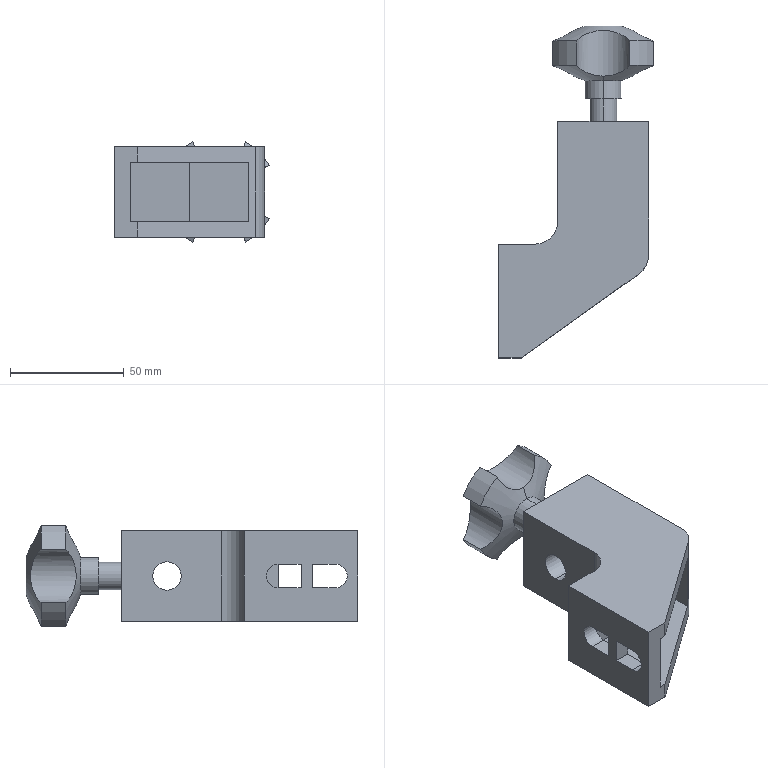Part | STEP file | Guide wheel mechanism revised.sldasm-Part-81 | 1 solid | 47 faces | box 68.12 x 146 x 44.24 mm | volume 143041 mm3 | plane 24 | cylinder 19 | cone 4 | commonest cylinder face diameters 24 x5 50 x4 10.5 x2 12 x2 12.5 x2 16 x2